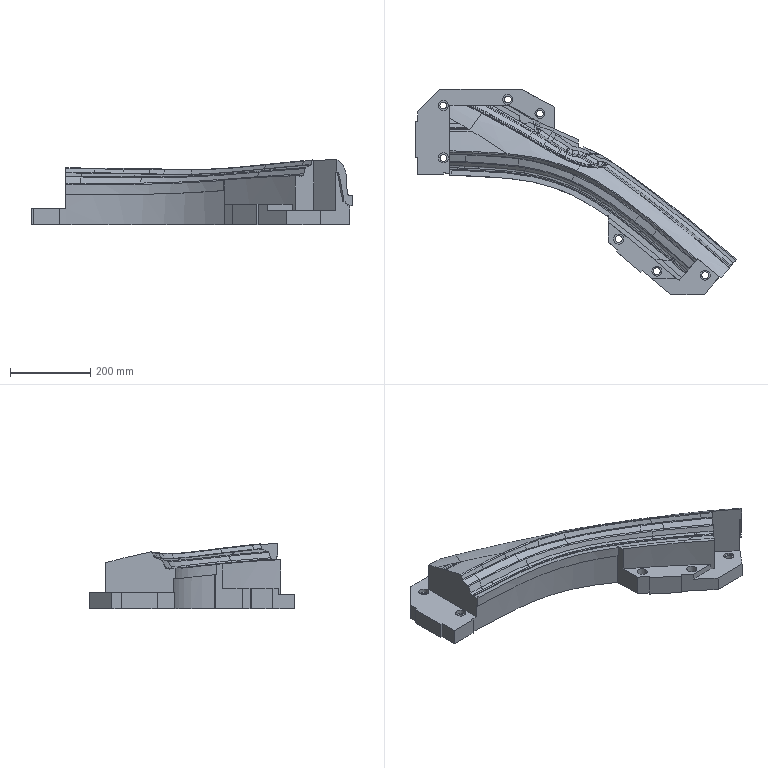Part | NX | features solid 2 | 1 solid | 287 faces | box 797.581 x 510 x 162.104 mm | volume 13203148 mm3 | spline 210 | plane 43 | cylinder 34 | commonest cylinder face diameters 17 x7 25 x7 4 x2 6.001 x2 8 x2 7130 x2